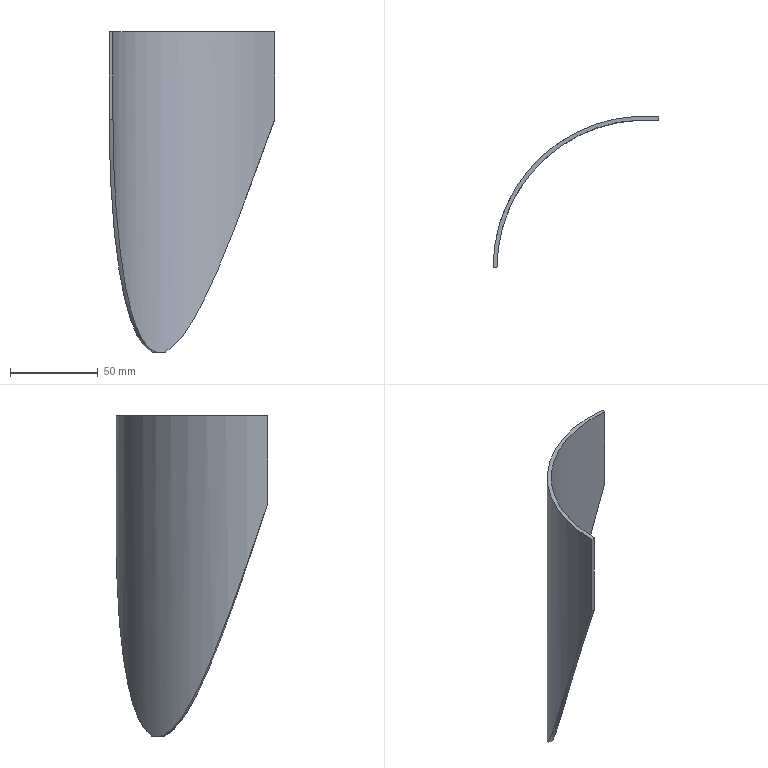Part | SolidWorks | 1 solid | 10 faces | box 94.546 x 86.364 x 182.8 mm | volume 42412 mm3 | plane 6 | cylinder 2 | spline 2 | commonest cylinder face diameters 168.269 x1 172.729 x1
STEP:
#1=CARTESIAN_POINT('',(83.843,-110.233,-985.22));
#2=VERTEX_POINT('',#1);
#3=CARTESIAN_POINT('',(83.843,-110.233,-984.858));
#4=VERTEX_POINT('',#3);
#5=CARTESIAN_POINT('',(83.843,-110.233,-985.22));
#6=DIRECTION('',(0.,0.,1.));
#7=VECTOR('',#6,1000.);
#8=LINE('',#5,#7);
#9=EDGE_CURVE('',#2,#4,#8,.T.);
#10=ORIENTED_EDGE('',*,*,#9,.F.);
#11=CARTESIAN_POINT('',(89.513,-104.991,-985.22));
#12=VERTEX_POINT('',#11);
#13=CARTESIAN_POINT('',(143.73,-169.327,-985.22));
#14=DIRECTION('',(0.,0.,-1.));
#15=DIRECTION('',(-0.7118,0.7024,0.));
#16=AXIS2_PLACEMENT_3D('',#13,#14,#15);
#17=CIRCLE('',#16,84.134);
#18=EDGE_CURVE('',#2,#12,#17,.T.);
#19=ORIENTED_EDGE('',*,*,#18,.T.);
#20=CARTESIAN_POINT('',(89.513,-104.991,-984.533));
#21=VERTEX_POINT('',#20);
#22=CARTESIAN_POINT('',(89.513,-104.991,-985.22));
#23=DIRECTION('',(0.,0.,1.));
#24=VECTOR('',#23,1000.);
#25=LINE('',#22,#24);
#26=EDGE_CURVE('',#12,#21,#25,.T.);
#27=ORIENTED_EDGE('',*,*,#26,.T.);
#28=CARTESIAN_POINT('',(151.7,-85.571,-852.42));
#29=VERTEX_POINT('',#28);
#30=CARTESIAN_POINT('',(151.7,-85.571,-852.42));
#31=CARTESIAN_POINT('',(150.614,-85.468,-855.388));
#32=CARTESIAN_POINT('',(149.545,-85.387,-858.323));
#33=CARTESIAN_POINT('',(147.407,-85.266,-864.21));
#34=CARTESIAN_POINT('',(146.334,-85.226,-867.173));
#35=CARTESIAN_POINT('',(144.195,-85.187,-873.077));
#36=CARTESIAN_POINT('',(143.126,-85.188,-876.029));
#37=CARTESIAN_POINT('',(140.983,-85.231,-881.932));
#38=CARTESIAN_POINT('',(139.91,-85.272,-884.884));
#39=CARTESIAN_POINT('',(136.678,-85.461,-893.73));
#40=CARTESIAN_POINT('',(134.508,-85.67,-899.62));
#41=CARTESIAN_POINT('',(130.095,-86.275,-911.365));
#42=CARTESIAN_POINT('',(127.853,-86.67,-917.219));
#43=CARTESIAN_POINT('',(124.395,-87.436,-925.949));
#44=CARTESIAN_POINT('',(123.226,-87.72,-928.851));
#45=CARTESIAN_POINT('',(121.442,-88.196,-933.183));
#46=CARTESIAN_POINT('',(120.842,-88.363,-934.624));
#47=CARTESIAN_POINT('',(119.629,-88.716,-937.501));
#48=CARTESIAN_POINT('',(119.018,-88.901,-938.933));
#49=CARTESIAN_POINT('',(118.089,-89.194,-941.078));
#50=CARTESIAN_POINT('',(117.778,-89.294,-941.792));
#51=CARTESIAN_POINT('',(117.152,-89.5,-943.216));
#52=CARTESIAN_POINT('',(116.838,-89.605,-943.926));
#53=CARTESIAN_POINT('',(115.887,-89.93,-946.056));
#54=CARTESIAN_POINT('',(115.243,-90.159,-947.475));
#55=CARTESIAN_POINT('',(113.942,-90.639,-950.291));
#56=CARTESIAN_POINT('',(113.282,-90.892,-951.691));
#57=CARTESIAN_POINT('',(111.94,-91.426,-954.479));
#58=CARTESIAN_POINT('',(111.258,-91.708,-955.867));
#59=CARTESIAN_POINT('',(109.868,-92.304,-958.619));
#60=CARTESIAN_POINT('',(109.161,-92.618,-959.985));
#61=CARTESIAN_POINT('',(107.716,-93.286,-962.691));
#62=CARTESIAN_POINT('',(106.978,-93.639,-964.033));
#63=CARTESIAN_POINT('',(105.465,-94.393,-966.68));
#64=CARTESIAN_POINT('',(104.69,-94.793,-967.986));
#65=CARTESIAN_POINT('',(103.096,-95.65,-970.553));
#66=CARTESIAN_POINT('',(102.276,-96.107,-971.813));
#67=CARTESIAN_POINT('',(100.581,-97.093,-974.266));
#68=CARTESIAN_POINT('',(99.706,-97.621,-975.458));
#69=CARTESIAN_POINT('',(97.884,-98.772,-977.745));
#70=CARTESIAN_POINT('',(96.94,-99.393,-978.838));
#71=CARTESIAN_POINT('',(94.965,-100.756,-980.866));
#72=CARTESIAN_POINT('',(93.934,-101.498,-981.799));
#73=CARTESIAN_POINT('',(91.783,-103.13,-983.404));
#74=CARTESIAN_POINT('',(90.662,-104.023,-984.073));
#75=CARTESIAN_POINT('',(89.513,-104.991,-984.533));
#76=B_SPLINE_CURVE_WITH_KNOTS('',3,(#30,#31,#32,#33,#34,#35,#36,#37,#38,#39,#40,#41,#42,#43,#44,#45,#46,#47,#48,#49,#50,#51,#52,#53,#54,#55,#56,#57,#58,#59,#60,#61,#62,#63,#64,#65,#66,#67,#68,#69,#70,#71,#72,#73,#74,#75),.UNSPECIFIED.,.F.,.F.,(4,2,2,2,2,2,2,2,2,2,2,2,2,2,2,2,2,2,2,2,2,2,4),(0.,0.0625,0.125,0.1875,0.25,0.375,0.5,0.5625,0.5938,0.625,0.6406,0.6563,0.6875,0.7188,0.75,0.7813,0.8125,0.8438,0.875,0.9063,0.9375,0.9688,1.),.UNSPECIFIED.);
#77=EDGE_CURVE('',#29,#21,#76,.T.);
#78=ORIENTED_EDGE('',*,*,#77,.F.);
#79=CARTESIAN_POINT('',(151.7,-85.571,-802.42));
#80=VERTEX_POINT('',#79);
#81=CARTESIAN_POINT('',(151.7,-85.571,-802.42));
#82=DIRECTION('',(0.,0.,-1.));
#83=VECTOR('',#82,1000.);
#84=LINE('',#81,#83);
#85=EDGE_CURVE('',#80,#29,#84,.T.);
#86=ORIENTED_EDGE('',*,*,#85,.F.);
#87=CARTESIAN_POINT('',(59.595,-169.327,-802.42));
#88=VERTEX_POINT('',#87);
#89=CARTESIAN_POINT('',(143.73,-169.327,-802.42));
#90=DIRECTION('',(0.,0.,1.));
#91=DIRECTION('',(0.09473,0.9955,0.));
#92=AXIS2_PLACEMENT_3D('',#89,#90,#91);
#93=CIRCLE('',#92,84.134);
#94=EDGE_CURVE('',#80,#88,#93,.T.);
#95=ORIENTED_EDGE('',*,*,#94,.T.);
#96=CARTESIAN_POINT('',(59.595,-169.327,-852.42));
#97=VERTEX_POINT('',#96);
#98=CARTESIAN_POINT('',(59.595,-169.327,-852.42));
#99=DIRECTION('',(0.,0.,1.));
#100=VECTOR('',#99,1000.);
#101=LINE('',#98,#100);
#102=EDGE_CURVE('',#97,#88,#101,.T.);
#103=ORIENTED_EDGE('',*,*,#102,.F.);
#104=CARTESIAN_POINT('',(83.843,-110.233,-984.858));
#105=CARTESIAN_POINT('',(83.303,-110.78,-984.687));
#106=CARTESIAN_POINT('',(82.781,-111.324,-984.458));
#107=CARTESIAN_POINT('',(81.775,-112.399,-983.902));
#108=CARTESIAN_POINT('',(81.293,-112.929,-983.575));
#109=CARTESIAN_POINT('',(79.905,-114.491,-982.478));
#110=CARTESIAN_POINT('',(79.06,-115.494,-981.595));
#111=CARTESIAN_POINT('',(77.509,-117.414,-979.643));
#112=CARTESIAN_POINT('',(76.802,-118.332,-978.575));
#113=CARTESIAN_POINT('',(75.491,-120.1,-976.326));
#114=CARTESIAN_POINT('',(74.888,-120.949,-975.145));
#115=CARTESIAN_POINT('',(73.763,-122.59,-972.708));
#116=CARTESIAN_POINT('',(73.241,-123.384,-971.451));
#117=CARTESIAN_POINT('',(72.261,-124.923,-968.89));
#118=CARTESIAN_POINT('',(71.803,-125.67,-967.584));
#119=CARTESIAN_POINT('',(70.938,-127.128,-964.932));
#120=CARTESIAN_POINT('',(70.532,-127.838,-963.589));
#121=CARTESIAN_POINT('',(69.762,-129.228,-960.874));
#122=CARTESIAN_POINT('',(69.397,-129.908,-959.501));
#123=CARTESIAN_POINT('',(68.705,-131.242,-956.737));
#124=CARTESIAN_POINT('',(68.378,-131.894,-955.348));
#125=CARTESIAN_POINT('',(67.753,-133.179,-952.548));
#126=CARTESIAN_POINT('',(67.455,-133.813,-951.134));
#127=CARTESIAN_POINT('',(66.603,-135.682,-946.886));
#128=CARTESIAN_POINT('',(66.089,-136.89,-944.029));
#129=CARTESIAN_POINT('',(64.671,-140.433,-935.396));
#130=CARTESIAN_POINT('',(63.892,-142.685,-929.572));
#131=CARTESIAN_POINT('',(62.563,-147.059,-917.849));
#132=CARTESIAN_POINT('',(62.015,-149.179,-911.951));
#133=CARTESIAN_POINT('',(61.101,-153.34,-900.111));
#134=CARTESIAN_POINT('',(60.734,-155.38,-894.17));
#135=CARTESIAN_POINT('',(60.156,-159.413,-882.267));
#136=CARTESIAN_POINT('',(59.945,-161.407,-876.302));
#137=CARTESIAN_POINT('',(59.77,-163.886,-868.844));
#138=CARTESIAN_POINT('',(59.739,-164.382,-867.35));
#139=CARTESIAN_POINT('',(59.687,-165.374,-864.36));
#140=CARTESIAN_POINT('',(59.665,-165.869,-862.865));
#141=CARTESIAN_POINT('',(59.613,-167.349,-858.395));
#142=CARTESIAN_POINT('',(59.596,-168.332,-855.424));
#143=CARTESIAN_POINT('',(59.595,-169.327,-852.42));
#144=B_SPLINE_CURVE_WITH_KNOTS('',3,(#104,#105,#106,#107,#108,#109,#110,#111,#112,#113,#114,#115,#116,#117,#118,#119,#120,#121,#122,#123,#124,#125,#126,#127,#128,#129,#130,#131,#132,#133,#134,#135,#136,#137,#138,#139,#140,#141,#142,#143),.UNSPECIFIED.,.F.,.F.,(4,2,2,2,2,2,2,2,2,2,2,2,2,2,2,2,2,2,2,4),(0.,0.01563,0.03125,0.0625,0.09375,0.125,0.1563,0.1875,0.2188,0.25,0.2813,0.3125,0.375,0.5,0.625,0.75,0.875,0.9063,0.9375,1.),.UNSPECIFIED.);
#145=EDGE_CURVE('',#4,#97,#144,.T.);
#146=ORIENTED_EDGE('',*,*,#145,.F.);
#147=EDGE_LOOP('',(#10,#19,#27,#78,#86,#95,#103,#146));
#148=FACE_OUTER_BOUND('',#147,.T.);
#149=CARTESIAN_POINT('',(143.73,-169.327,-802.42));
#150=DIRECTION('',(0.,0.,-1.));
#151=DIRECTION('',(-1.,0.,0.));
#152=AXIS2_PLACEMENT_3D('',#149,#150,#151);
#153=CYLINDRICAL_SURFACE('',#152,84.134);
#154=ADVANCED_FACE('',(#148),#153,.F.);
#155=CARTESIAN_POINT('',(82.255,-108.666,-985.22));
#156=VERTEX_POINT('',#155);
#157=CARTESIAN_POINT('',(82.255,-108.666,-985.22));
#158=DIRECTION('',(0.7118,-0.7024,0.));
#159=VECTOR('',#158,1000.);
#160=LINE('',#157,#159);
#161=EDGE_CURVE('',#156,#2,#160,.T.);
#162=ORIENTED_EDGE('',*,*,#161,.T.);
#163=ORIENTED_EDGE('',*,*,#9,.T.);
#164=CARTESIAN_POINT('',(82.255,-108.666,-984.858));
#165=VERTEX_POINT('',#164);
#166=CARTESIAN_POINT('',(83.049,-109.45,-984.858));
#167=DIRECTION('',(-0.7118,0.7024,0.));
#168=VECTOR('',#167,1000.);
#169=LINE('',#166,#168);
#170=EDGE_CURVE('',#4,#165,#169,.T.);
#171=ORIENTED_EDGE('',*,*,#170,.T.);
#172=CARTESIAN_POINT('',(82.255,-108.666,-984.858));
#173=DIRECTION('',(0.,0.,-1.));
#174=VECTOR('',#173,1000.);
#175=LINE('',#172,#174);
#176=EDGE_CURVE('',#165,#156,#175,.T.);
#177=ORIENTED_EDGE('',*,*,#176,.T.);
#178=EDGE_LOOP('',(#162,#163,#171,#177));
#179=FACE_OUTER_BOUND('',#178,.T.);
#180=CARTESIAN_POINT('',(83.049,-109.45,-985.039));
#181=DIRECTION('',(0.7024,0.7118,0.));
#182=DIRECTION('',(0.,0.,-1.));
#183=AXIS2_PLACEMENT_3D('',#180,#181,#182);
#184=PLANE('',#183);
#185=ADVANCED_FACE('',(#179),#184,.F.);
#186=CARTESIAN_POINT('',(88.076,-103.286,-985.22));
#187=VERTEX_POINT('',#186);
#188=CARTESIAN_POINT('',(89.513,-104.991,-985.22));
#189=DIRECTION('',(-0.6444,0.7647,0.));
#190=VECTOR('',#189,1000.);
#191=LINE('',#188,#190);
#192=EDGE_CURVE('',#12,#187,#191,.T.);
#193=ORIENTED_EDGE('',*,*,#192,.F.);
#194=ORIENTED_EDGE('',*,*,#18,.F.);
#195=ORIENTED_EDGE('',*,*,#161,.F.);
#196=CARTESIAN_POINT('',(143.73,-169.327,-985.22));
#197=DIRECTION('',(0.,0.,1.));
#198=DIRECTION('',(-0.6444,0.7647,0.));
#199=AXIS2_PLACEMENT_3D('',#196,#197,#198);
#200=CIRCLE('',#199,86.364);
#201=EDGE_CURVE('',#187,#156,#200,.T.);
#202=ORIENTED_EDGE('',*,*,#201,.F.);
#203=EDGE_LOOP('',(#193,#194,#195,#202));
#204=FACE_OUTER_BOUND('',#203,.T.);
#205=CARTESIAN_POINT('',(85.86,-106.728,-985.22));
#206=DIRECTION('',(0.,0.,1.));
#207=DIRECTION('',(0.7024,0.7118,0.));
#208=AXIS2_PLACEMENT_3D('',#205,#206,#207);
#209=PLANE('',#208);
#210=ADVANCED_FACE('',(#204),#209,.F.);
#211=CARTESIAN_POINT('',(88.076,-103.286,-984.533));
#212=VERTEX_POINT('',#211);
#213=CARTESIAN_POINT('',(88.794,-104.138,-984.533));
#214=DIRECTION('',(0.6444,-0.7647,0.));
#215=VECTOR('',#214,1000.);
#216=LINE('',#213,#215);
#217=EDGE_CURVE('',#212,#21,#216,.T.);
#218=ORIENTED_EDGE('',*,*,#217,.T.);
#219=ORIENTED_EDGE('',*,*,#26,.F.);
#220=ORIENTED_EDGE('',*,*,#192,.T.);
#221=CARTESIAN_POINT('',(88.076,-103.286,-985.22));
#222=DIRECTION('',(0.,0.,1.));
#223=VECTOR('',#222,1000.);
#224=LINE('',#221,#223);
#225=EDGE_CURVE('',#187,#212,#224,.T.);
#226=ORIENTED_EDGE('',*,*,#225,.T.);
#227=EDGE_LOOP('',(#218,#219,#220,#226));
#228=FACE_OUTER_BOUND('',#227,.T.);
#229=CARTESIAN_POINT('',(88.794,-104.138,-984.877));
#230=DIRECTION('',(0.7647,0.6444,0.));
#231=DIRECTION('',(0.,0.,-1.));
#232=AXIS2_PLACEMENT_3D('',#229,#230,#231);
#233=PLANE('',#232);
#234=ADVANCED_FACE('',(#228),#233,.T.);
#235=CARTESIAN_POINT('',(151.911,-83.351,-852.42));
#236=VERTEX_POINT('',#235);
#237=CARTESIAN_POINT('',(151.805,-84.461,-852.42));
#238=DIRECTION('',(0.09473,0.9955,0.));
#239=VECTOR('',#238,1000.);
#240=LINE('',#237,#239);
#241=EDGE_CURVE('',#29,#236,#240,.T.);
#242=ORIENTED_EDGE('',*,*,#241,.F.);
#243=ORIENTED_EDGE('',*,*,#77,.T.);
#244=ORIENTED_EDGE('',*,*,#217,.F.);
#245=CARTESIAN_POINT('',(88.076,-103.286,-984.533));
#246=CARTESIAN_POINT('',(89.234,-102.31,-984.082));
#247=CARTESIAN_POINT('',(90.367,-101.407,-983.427));
#248=CARTESIAN_POINT('',(92.548,-99.749,-981.852));
#249=CARTESIAN_POINT('',(93.596,-98.993,-980.935));
#250=CARTESIAN_POINT('',(95.609,-97.601,-978.936));
#251=CARTESIAN_POINT('',(96.573,-96.965,-977.856));
#252=CARTESIAN_POINT('',(98.436,-95.785,-975.591));
#253=CARTESIAN_POINT('',(99.332,-95.241,-974.408));
#254=CARTESIAN_POINT('',(101.068,-94.228,-971.972));
#255=CARTESIAN_POINT('',(101.909,-93.758,-970.719));
#256=CARTESIAN_POINT('',(103.545,-92.875,-968.166));
#257=CARTESIAN_POINT('',(104.34,-92.463,-966.864));
#258=CARTESIAN_POINT('',(105.893,-91.687,-964.225));
#259=CARTESIAN_POINT('',(106.652,-91.322,-962.887));
#260=CARTESIAN_POINT('',(108.137,-90.634,-960.186));
#261=CARTESIAN_POINT('',(108.863,-90.309,-958.823));
#262=CARTESIAN_POINT('',(110.292,-89.694,-956.073));
#263=CARTESIAN_POINT('',(110.993,-89.404,-954.687));
#264=CARTESIAN_POINT('',(112.374,-88.852,-951.9));
#265=CARTESIAN_POINT('',(113.052,-88.591,-950.499));
#266=CARTESIAN_POINT('',(114.391,-88.096,-947.684));
#267=CARTESIAN_POINT('',(115.052,-87.86,-946.266));
#268=CARTESIAN_POINT('',(116.357,-87.412,-943.421));
#269=CARTESIAN_POINT('',(117.,-87.2,-941.998));
#270=CARTESIAN_POINT('',(118.274,-86.797,-939.135));
#271=CARTESIAN_POINT('',(118.903,-86.605,-937.702));
#272=CARTESIAN_POINT('',(120.15,-86.241,-934.821));
#273=CARTESIAN_POINT('',(120.768,-86.068,-933.378));
#274=CARTESIAN_POINT('',(122.603,-85.577,-929.04));
#275=CARTESIAN_POINT('',(123.807,-85.283,-926.133));
#276=CARTESIAN_POINT('',(127.366,-84.492,-917.386));
#277=CARTESIAN_POINT('',(129.673,-84.083,-911.519));
#278=CARTESIAN_POINT('',(134.216,-83.458,-899.747));
#279=CARTESIAN_POINT('',(136.45,-83.241,-893.84));
#280=CARTESIAN_POINT('',(140.885,-82.981,-882.015));
#281=CARTESIAN_POINT('',(143.086,-82.937,-876.093));
#282=CARTESIAN_POINT('',(146.388,-82.996,-867.212));
#283=CARTESIAN_POINT('',(147.492,-83.037,-864.242));
#284=CARTESIAN_POINT('',(149.694,-83.162,-858.337));
#285=CARTESIAN_POINT('',(150.794,-83.245,-855.394));
#286=CARTESIAN_POINT('',(151.911,-83.351,-852.42));
#287=B_SPLINE_CURVE_WITH_KNOTS('',3,(#245,#246,#247,#248,#249,#250,#251,#252,#253,#254,#255,#256,#257,#258,#259,#260,#261,#262,#263,#264,#265,#266,#267,#268,#269,#270,#271,#272,#273,#274,#275,#276,#277,#278,#279,#280,#281,#282,#283,#284,#285,#286),.UNSPECIFIED.,.F.,.F.,(4,2,2,2,2,2,2,2,2,2,2,2,2,2,2,2,2,2,2,2,4),(0.,0.03125,0.0625,0.09375,0.125,0.1563,0.1875,0.2188,0.25,0.2813,0.3125,0.3438,0.375,0.4063,0.4375,0.5,0.625,0.75,0.875,0.9375,1.),.UNSPECIFIED.);
#288=EDGE_CURVE('',#212,#236,#287,.T.);
#289=ORIENTED_EDGE('',*,*,#288,.T.);
#290=EDGE_LOOP('',(#242,#243,#244,#289));
#291=FACE_OUTER_BOUND('',#290,.T.);
#292=CARTESIAN_POINT('',(152.469,-83.136,-851.006));
#293=CARTESIAN_POINT('',(152.376,-84.053,-851.006));
#294=CARTESIAN_POINT('',(152.283,-84.971,-851.006));
#295=CARTESIAN_POINT('',(152.19,-85.889,-851.006));
#296=CARTESIAN_POINT('',(152.292,-83.118,-851.477));
#297=CARTESIAN_POINT('',(152.201,-84.036,-851.477));
#298=CARTESIAN_POINT('',(152.109,-84.954,-851.477));
#299=CARTESIAN_POINT('',(152.018,-85.871,-851.477));
#300=CARTESIAN_POINT('',(150.752,-82.967,-855.56));
#301=CARTESIAN_POINT('',(150.677,-83.886,-855.56));
#302=CARTESIAN_POINT('',(150.603,-84.806,-855.56));
#303=CARTESIAN_POINT('',(150.528,-85.725,-855.56));
#304=CARTESIAN_POINT('',(147.847,-82.758,-863.317));
#305=CARTESIAN_POINT('',(147.803,-83.68,-863.317));
#306=CARTESIAN_POINT('',(147.759,-84.601,-863.317));
#307=CARTESIAN_POINT('',(147.716,-85.523,-863.317));
#308=CARTESIAN_POINT('',(143.616,-82.66,-874.671));
#309=CARTESIAN_POINT('',(143.617,-83.583,-874.671));
#310=CARTESIAN_POINT('',(143.618,-84.505,-874.671));
#311=CARTESIAN_POINT('',(143.619,-85.428,-874.671));
#312=CARTESIAN_POINT('',(139.544,-82.766,-885.568));
#313=CARTESIAN_POINT('',(139.589,-83.687,-885.568));
#314=CARTESIAN_POINT('',(139.633,-84.609,-885.568));
#315=CARTESIAN_POINT('',(139.678,-85.53,-885.568));
#316=CARTESIAN_POINT('',(135.85,-83.03,-895.364));
#317=CARTESIAN_POINT('',(135.934,-83.949,-895.364));
#318=CARTESIAN_POINT('',(136.018,-84.867,-895.364));
#319=CARTESIAN_POINT('',(136.102,-85.786,-895.364));
#320=CARTESIAN_POINT('',(132.603,-83.392,-903.857));
#321=CARTESIAN_POINT('',(132.721,-84.307,-903.857));
#322=CARTESIAN_POINT('',(132.84,-85.222,-903.857));
#323=CARTESIAN_POINT('',(132.958,-86.137,-903.857));
#324=CARTESIAN_POINT('',(129.554,-83.844,-911.696));
#325=CARTESIAN_POINT('',(129.705,-84.754,-911.696));
#326=CARTESIAN_POINT('',(129.856,-85.664,-911.696));
#327=CARTESIAN_POINT('',(130.007,-86.575,-911.696));
#328=CARTESIAN_POINT('',(126.746,-84.36,-918.768));
#329=CARTESIAN_POINT('',(126.927,-85.265,-918.768));
#330=CARTESIAN_POINT('',(127.108,-86.169,-918.768));
#331=CARTESIAN_POINT('',(127.289,-87.074,-918.768));
#332=CARTESIAN_POINT('',(124.157,-84.921,-925.14));
#333=CARTESIAN_POINT('',(124.366,-85.82,-925.14));
#334=CARTESIAN_POINT('',(124.574,-86.718,-925.14));
#335=CARTESIAN_POINT('',(124.782,-87.617,-925.14));
#336=CARTESIAN_POINT('',(121.795,-85.506,-930.81));
#337=CARTESIAN_POINT('',(122.028,-86.399,-930.81));
#338=CARTESIAN_POINT('',(122.262,-87.291,-930.81));
#339=CARTESIAN_POINT('',(122.496,-88.183,-930.81));
#340=CARTESIAN_POINT('',(119.681,-86.09,-935.751));
#341=CARTESIAN_POINT('',(119.938,-86.976,-935.751));
#342=CARTESIAN_POINT('',(120.194,-87.862,-935.751));
#343=CARTESIAN_POINT('',(120.45,-88.748,-935.751));
#344=CARTESIAN_POINT('',(117.732,-86.678,-940.192));
#345=CARTESIAN_POINT('',(118.009,-87.558,-940.192));
#346=CARTESIAN_POINT('',(118.286,-88.438,-940.192));
#347=CARTESIAN_POINT('',(118.562,-89.318,-940.192));
#348=CARTESIAN_POINT('',(115.769,-87.321,-944.539));
#349=CARTESIAN_POINT('',(116.066,-88.194,-944.539));
#350=CARTESIAN_POINT('',(116.364,-89.067,-944.539));
#351=CARTESIAN_POINT('',(116.662,-89.94,-944.539));
#352=CARTESIAN_POINT('',(113.692,-88.057,-948.986));
#353=CARTESIAN_POINT('',(114.012,-88.923,-948.986));
#354=CARTESIAN_POINT('',(114.332,-89.788,-948.986));
#355=CARTESIAN_POINT('',(114.652,-90.653,-948.986));
#356=CARTESIAN_POINT('',(111.544,-88.883,-953.407));
#357=CARTESIAN_POINT('',(111.887,-89.739,-953.407));
#358=CARTESIAN_POINT('',(112.23,-90.596,-953.407));
#359=CARTESIAN_POINT('',(112.572,-91.452,-953.407));
#360=CARTESIAN_POINT('',(109.338,-89.8,-957.742));
#361=CARTESIAN_POINT('',(109.704,-90.647,-957.742));
#362=CARTESIAN_POINT('',(110.07,-91.494,-957.742));
#363=CARTESIAN_POINT('',(110.436,-92.341,-957.742));
#364=CARTESIAN_POINT('',(107.093,-90.809,-961.921));
#365=CARTESIAN_POINT('',(107.483,-91.645,-961.921));
#366=CARTESIAN_POINT('',(107.873,-92.481,-961.921));
#367=CARTESIAN_POINT('',(108.263,-93.317,-961.921));
#368=CARTESIAN_POINT('',(104.829,-91.905,-965.874));
#369=CARTESIAN_POINT('',(105.243,-92.729,-965.874));
#370=CARTESIAN_POINT('',(105.657,-93.554,-965.874));
#371=CARTESIAN_POINT('',(106.071,-94.378,-965.874));
#372=CARTESIAN_POINT('',(102.594,-93.069,-969.5));
#373=CARTESIAN_POINT('',(103.031,-93.881,-969.5));
#374=CARTESIAN_POINT('',(103.469,-94.693,-969.5));
#375=CARTESIAN_POINT('',(103.907,-95.505,-969.5));
#376=CARTESIAN_POINT('',(100.388,-94.3,-972.787));
#377=CARTESIAN_POINT('',(100.85,-95.099,-972.787));
#378=CARTESIAN_POINT('',(101.311,-95.898,-972.787));
#379=CARTESIAN_POINT('',(101.773,-96.697,-972.787));
#380=CARTESIAN_POINT('',(98.152,-95.636,-975.803));
#381=CARTESIAN_POINT('',(98.637,-96.421,-975.803));
#382=CARTESIAN_POINT('',(99.122,-97.205,-975.803));
#383=CARTESIAN_POINT('',(99.607,-97.99,-975.803));
#384=CARTESIAN_POINT('',(95.801,-97.141,-978.599));
#385=CARTESIAN_POINT('',(96.311,-97.909,-978.599));
#386=CARTESIAN_POINT('',(96.821,-98.678,-978.599));
#387=CARTESIAN_POINT('',(97.331,-99.446,-978.599));
#388=CARTESIAN_POINT('',(93.314,-98.851,-981.099));
#389=CARTESIAN_POINT('',(93.851,-99.601,-981.099));
#390=CARTESIAN_POINT('',(94.388,-100.351,-981.099));
#391=CARTESIAN_POINT('',(94.925,-101.102,-981.099));
#392=CARTESIAN_POINT('',(90.661,-100.822,-983.191));
#393=CARTESIAN_POINT('',(91.226,-101.551,-983.191));
#394=CARTESIAN_POINT('',(91.791,-102.281,-983.191));
#395=CARTESIAN_POINT('',(92.356,-103.01,-983.191));
#396=CARTESIAN_POINT('',(88.473,-102.586,-984.365));
#397=CARTESIAN_POINT('',(89.061,-103.297,-984.365));
#398=CARTESIAN_POINT('',(89.65,-104.007,-984.365));
#399=CARTESIAN_POINT('',(90.238,-104.718,-984.365));
#400=CARTESIAN_POINT('',(87.155,-103.716,-984.802));
#401=CARTESIAN_POINT('',(87.757,-104.414,-984.802));
#402=CARTESIAN_POINT('',(88.36,-105.113,-984.802));
#403=CARTESIAN_POINT('',(88.962,-105.811,-984.802));
#404=CARTESIAN_POINT('',(86.775,-104.046,-984.906));
#405=CARTESIAN_POINT('',(87.382,-104.741,-984.906));
#406=CARTESIAN_POINT('',(87.988,-105.436,-984.906));
#407=CARTESIAN_POINT('',(88.595,-106.132,-984.906));
#408=B_SPLINE_SURFACE_WITH_KNOTS('',3,3,((#292,#293,#294,#295),(#296,#297,#298,#299),(#300,#301,#302,#303),(#304,#305,#306,#307),(#308,#309,#310,#311),(#312,#313,#314,#315),(#316,#317,#318,#319),(#320,#321,#322,#323),(#324,#325,#326,#327),(#328,#329,#330,#331),(#332,#333,#334,#335),(#336,#337,#338,#339),(#340,#341,#342,#343),(#344,#345,#346,#347),(#348,#349,#350,#351),(#352,#353,#354,#355),(#356,#357,#358,#359),(#360,#361,#362,#363),(#364,#365,#366,#367),(#368,#369,#370,#371),(#372,#373,#374,#375),(#376,#377,#378,#379),(#380,#381,#382,#383),(#384,#385,#386,#387),(#388,#389,#390,#391),(#392,#393,#394,#395),(#396,#397,#398,#399),(#400,#401,#402,#403),(#404,#405,#406,#407)),.UNSPECIFIED.,.F.,.F.,.F.,(4,1,1,1,1,1,1,1,1,1,1,1,1,1,1,1,1,1,1,1,1,1,1,1,1,1,4),(4,4),(-0.005438,0.,0.04167,0.08333,0.125,0.1667,0.2083,0.25,0.2917,0.3333,0.375,0.4167,0.4583,0.5,0.5417,0.5833,0.625,0.6667,0.7083,0.75,0.7917,0.8333,0.875,0.9167,0.9583,1.,1.017),(-0.00003046,1.),.UNSPECIFIED.);
#409=ADVANCED_FACE('',(#291),#408,.F.);
#410=CARTESIAN_POINT('',(151.911,-83.351,-802.42));
#411=VERTEX_POINT('',#410);
#412=CARTESIAN_POINT('',(151.911,-83.351,-802.42));
#413=DIRECTION('',(-0.09473,-0.9955,0.));
#414=VECTOR('',#413,1000.);
#415=LINE('',#412,#414);
#416=EDGE_CURVE('',#411,#80,#415,.T.);
#417=ORIENTED_EDGE('',*,*,#416,.T.);
#418=ORIENTED_EDGE('',*,*,#85,.T.);
#419=ORIENTED_EDGE('',*,*,#241,.T.);
#420=CARTESIAN_POINT('',(151.911,-83.351,-852.42));
#421=DIRECTION('',(0.,0.,1.));
#422=VECTOR('',#421,1000.);
#423=LINE('',#420,#422);
#424=EDGE_CURVE('',#236,#411,#423,.T.);
#425=ORIENTED_EDGE('',*,*,#424,.T.);
#426=EDGE_LOOP('',(#417,#418,#419,#425));
#427=FACE_OUTER_BOUND('',#426,.T.);
#428=CARTESIAN_POINT('',(151.805,-84.461,-827.42));
#429=DIRECTION('',(0.9955,-0.09473,0.));
#430=DIRECTION('',(0.,0.,-1.));
#431=AXIS2_PLACEMENT_3D('',#428,#429,#430);
#432=PLANE('',#431);
#433=ADVANCED_FACE('',(#427),#432,.T.);
#434=CARTESIAN_POINT('',(57.365,-169.327,-802.42));
#435=VERTEX_POINT('',#434);
#436=CARTESIAN_POINT('',(57.365,-169.327,-802.42));
#437=DIRECTION('',(1.,0.,0.));
#438=VECTOR('',#437,1000.);
#439=LINE('',#436,#438);
#440=EDGE_CURVE('',#435,#88,#439,.T.);
#441=ORIENTED_EDGE('',*,*,#440,.T.);
#442=ORIENTED_EDGE('',*,*,#94,.F.);
#443=ORIENTED_EDGE('',*,*,#416,.F.);
#444=CARTESIAN_POINT('',(143.73,-169.327,-802.42));
#445=DIRECTION('',(0.,0.,-1.));
#446=DIRECTION('',(-1.,0.,0.));
#447=AXIS2_PLACEMENT_3D('',#444,#445,#446);
#448=CIRCLE('',#447,86.364);
#449=EDGE_CURVE('',#435,#411,#448,.T.);
#450=ORIENTED_EDGE('',*,*,#449,.F.);
#451=EDGE_LOOP('',(#441,#442,#443,#450));
#452=FACE_OUTER_BOUND('',#451,.T.);
#453=CARTESIAN_POINT('',(86.375,-106.256,-802.42));
#454=DIRECTION('',(0.,0.,1.));
#455=DIRECTION('',(0.,1.,0.));
#456=AXIS2_PLACEMENT_3D('',#453,#454,#455);
#457=PLANE('',#456);
#458=ADVANCED_FACE('',(#452),#457,.T.);
#459=CARTESIAN_POINT('',(57.365,-169.327,-852.42));
#460=VERTEX_POINT('',#459);
#461=CARTESIAN_POINT('',(58.48,-169.327,-852.42));
#462=DIRECTION('',(1.,0.,0.));
#463=VECTOR('',#462,1000.);
#464=LINE('',#461,#463);
#465=EDGE_CURVE('',#460,#97,#464,.T.);
#466=ORIENTED_EDGE('',*,*,#465,.T.);
#467=ORIENTED_EDGE('',*,*,#102,.T.);
#468=ORIENTED_EDGE('',*,*,#440,.F.);
#469=CARTESIAN_POINT('',(57.365,-169.327,-802.42));
#470=DIRECTION('',(0.,0.,-1.));
#471=VECTOR('',#470,1000.);
#472=LINE('',#469,#471);
#473=EDGE_CURVE('',#435,#460,#472,.T.);
#474=ORIENTED_EDGE('',*,*,#473,.T.);
#475=EDGE_LOOP('',(#466,#467,#468,#474));
#476=FACE_OUTER_BOUND('',#475,.T.);
#477=CARTESIAN_POINT('',(58.48,-169.327,-827.42));
#478=DIRECTION('',(0.,1.,0.));
#479=DIRECTION('',(0.,0.,-1.));
#480=AXIS2_PLACEMENT_3D('',#477,#478,#479);
#481=PLANE('',#480);
#482=ADVANCED_FACE('',(#476),#481,.F.);
#483=ORIENTED_EDGE('',*,*,#170,.F.);
#484=ORIENTED_EDGE('',*,*,#145,.T.);
#485=ORIENTED_EDGE('',*,*,#465,.F.);
#486=CARTESIAN_POINT('',(57.365,-169.327,-852.42));
#487=CARTESIAN_POINT('',(57.366,-168.303,-855.432));
#488=CARTESIAN_POINT('',(57.383,-167.291,-858.413));
#489=CARTESIAN_POINT('',(57.437,-165.767,-862.898));
#490=CARTESIAN_POINT('',(57.46,-165.257,-864.396));
#491=CARTESIAN_POINT('',(57.514,-164.236,-867.396));
#492=CARTESIAN_POINT('',(57.546,-163.725,-868.894));
#493=CARTESIAN_POINT('',(57.727,-161.172,-876.374));
#494=CARTESIAN_POINT('',(57.945,-159.12,-882.357));
#495=CARTESIAN_POINT('',(58.542,-154.967,-894.294));
#496=CARTESIAN_POINT('',(58.92,-152.867,-900.251));
#497=CARTESIAN_POINT('',(59.865,-148.583,-912.121));
#498=CARTESIAN_POINT('',(60.431,-146.399,-918.034));
#499=CARTESIAN_POINT('',(61.46,-143.023,-926.844));
#500=CARTESIAN_POINT('',(61.833,-141.88,-929.77));
#501=CARTESIAN_POINT('',(62.651,-139.55,-935.595));
#502=CARTESIAN_POINT('',(63.096,-138.364,-938.495));
#503=CARTESIAN_POINT('',(64.072,-135.933,-944.255));
#504=CARTESIAN_POINT('',(64.603,-134.69,-947.113));
#505=CARTESIAN_POINT('',(65.482,-132.767,-951.363));
#506=CARTESIAN_POINT('',(65.79,-132.115,-952.776));
#507=CARTESIAN_POINT('',(66.434,-130.794,-955.573));
#508=CARTESIAN_POINT('',(66.773,-130.122,-956.963));
#509=CARTESIAN_POINT('',(67.844,-128.065,-961.105));
#510=CARTESIAN_POINT('',(68.63,-126.642,-963.821));
#511=CARTESIAN_POINT('',(69.968,-124.396,-967.784));
#512=CARTESIAN_POINT('',(70.44,-123.629,-969.085));
#513=CARTESIAN_POINT('',(71.448,-122.05,-971.632));
#514=CARTESIAN_POINT('',(71.986,-121.236,-972.881));
#515=CARTESIAN_POINT('',(73.142,-119.555,-975.299));
#516=CARTESIAN_POINT('',(73.761,-118.686,-976.469));
#517=CARTESIAN_POINT('',(75.105,-116.879,-978.692));
#518=CARTESIAN_POINT('',(75.83,-115.942,-979.746));
#519=CARTESIAN_POINT('',(77.413,-113.987,-981.666));
#520=CARTESIAN_POINT('',(78.273,-112.968,-982.531));
#521=CARTESIAN_POINT('',(79.681,-111.387,-983.604));
#522=CARTESIAN_POINT('',(80.169,-110.851,-983.924));
#523=CARTESIAN_POINT('',(81.185,-109.766,-984.467));
#524=CARTESIAN_POINT('',(81.712,-109.217,-984.69));
#525=CARTESIAN_POINT('',(82.255,-108.666,-984.858));
#526=B_SPLINE_CURVE_WITH_KNOTS('',3,(#486,#487,#488,#489,#490,#491,#492,#493,#494,#495,#496,#497,#498,#499,#500,#501,#502,#503,#504,#505,#506,#507,#508,#509,#510,#511,#512,#513,#514,#515,#516,#517,#518,#519,#520,#521,#522,#523,#524,#525),.UNSPECIFIED.,.F.,.F.,(4,2,2,2,2,2,2,2,2,2,2,2,2,2,2,2,2,2,2,4),(0.,0.0625,0.09375,0.125,0.25,0.375,0.5,0.5625,0.625,0.6875,0.7187,0.75,0.8125,0.8437,0.875,0.9062,0.9375,0.9687,0.9844,1.),.UNSPECIFIED.);
#527=EDGE_CURVE('',#460,#165,#526,.T.);
#528=ORIENTED_EDGE('',*,*,#527,.T.);
#529=EDGE_LOOP('',(#483,#484,#485,#528));
#530=FACE_OUTER_BOUND('',#529,.T.);
#531=CARTESIAN_POINT('',(83.127,-107.419,-985.112));
#532=CARTESIAN_POINT('',(83.772,-108.078,-985.112));
#533=CARTESIAN_POINT('',(84.417,-108.737,-985.112));
#534=CARTESIAN_POINT('',(85.063,-109.396,-985.112));
#535=CARTESIAN_POINT('',(82.765,-107.774,-985.05));
#536=CARTESIAN_POINT('',(83.414,-108.429,-985.05));
#537=CARTESIAN_POINT('',(84.063,-109.084,-985.05));
#538=CARTESIAN_POINT('',(84.712,-109.74,-985.05));
#539=CARTESIAN_POINT('',(81.563,-108.971,-984.762));
#540=CARTESIAN_POINT('',(82.225,-109.614,-984.762));
#541=CARTESIAN_POINT('',(82.887,-110.257,-984.762));
#542=CARTESIAN_POINT('',(83.548,-110.899,-984.762));
#543=CARTESIAN_POINT('',(79.664,-110.978,-983.84));
#544=CARTESIAN_POINT('',(80.346,-111.599,-983.84));
#545=CARTESIAN_POINT('',(81.028,-112.22,-983.84));
#546=CARTESIAN_POINT('',(81.71,-112.841,-983.84));
#547=CARTESIAN_POINT('',(77.511,-113.437,-982.042));
#548=CARTESIAN_POINT('',(78.216,-114.032,-982.042));
#549=CARTESIAN_POINT('',(78.921,-114.627,-982.042));
#550=CARTESIAN_POINT('',(79.626,-115.222,-982.042));
#551=CARTESIAN_POINT('',(75.614,-115.77,-979.785));
#552=CARTESIAN_POINT('',(76.339,-116.34,-979.785));
#553=CARTESIAN_POINT('',(77.065,-116.91,-979.785));
#554=CARTESIAN_POINT('',(77.79,-117.48,-979.785));
#555=CARTESIAN_POINT('',(73.908,-118.018,-977.155));
#556=CARTESIAN_POINT('',(74.651,-118.564,-977.155));
#557=CARTESIAN_POINT('',(75.394,-119.11,-977.155));
#558=CARTESIAN_POINT('',(76.138,-119.656,-977.155));
#559=CARTESIAN_POINT('',(72.372,-120.178,-974.239));
#560=CARTESIAN_POINT('',(73.132,-120.702,-974.239));
#561=CARTESIAN_POINT('',(73.891,-121.225,-974.239));
#562=CARTESIAN_POINT('',(74.651,-121.748,-974.239));
#563=CARTESIAN_POINT('',(70.979,-122.267,-971.089));
#564=CARTESIAN_POINT('',(71.754,-122.768,-971.089));
#565=CARTESIAN_POINT('',(72.528,-123.269,-971.089));
#566=CARTESIAN_POINT('',(73.303,-123.77,-971.089));
#567=CARTESIAN_POINT('',(69.716,-124.282,-967.764));
#568=CARTESIAN_POINT('',(70.504,-124.762,-967.764));
#569=CARTESIAN_POINT('',(71.292,-125.242,-967.764));
#570=CARTESIAN_POINT('',(72.08,-125.721,-967.764));
#571=CARTESIAN_POINT('',(68.567,-126.229,-964.305));
#572=CARTESIAN_POINT('',(69.367,-126.688,-964.305));
#573=CARTESIAN_POINT('',(70.167,-127.147,-964.305));
#574=CARTESIAN_POINT('',(70.968,-127.605,-964.305));
#575=CARTESIAN_POINT('',(67.532,-128.089,-960.789));
#576=CARTESIAN_POINT('',(68.343,-128.528,-960.789));
#577=CARTESIAN_POINT('',(69.154,-128.967,-960.789));
#578=CARTESIAN_POINT('',(69.966,-129.406,-960.789));
#579=CARTESIAN_POINT('',(66.605,-129.851,-957.28));
#580=CARTESIAN_POINT('',(67.426,-130.272,-957.28));
#581=CARTESIAN_POINT('',(68.247,-130.692,-957.28));
#582=CARTESIAN_POINT('',(69.068,-131.112,-957.28));
#583=CARTESIAN_POINT('',(65.759,-131.551,-953.743));
#584=CARTESIAN_POINT('',(66.589,-131.954,-953.743));
#585=CARTESIAN_POINT('',(67.419,-132.356,-953.743));
#586=CARTESIAN_POINT('',(68.249,-132.758,-953.743));
#587=CARTESIAN_POINT('',(64.973,-133.219,-950.138));
#588=CARTESIAN_POINT('',(65.812,-133.603,-950.138));
#589=CARTESIAN_POINT('',(66.65,-133.987,-950.138));
#590=CARTESIAN_POINT('',(67.489,-134.372,-950.138));
#591=CARTESIAN_POINT('',(64.254,-134.832,-946.528));
#592=CARTESIAN_POINT('',(65.1,-135.199,-946.528));
#593=CARTESIAN_POINT('',(65.946,-135.567,-946.528));
#594=CARTESIAN_POINT('',(66.792,-135.934,-946.528));
#595=CARTESIAN_POINT('',(63.592,-136.4,-942.915));
#596=CARTESIAN_POINT('',(64.445,-136.75,-942.915));
#597=CARTESIAN_POINT('',(65.298,-137.101,-942.915));
#598=CARTESIAN_POINT('',(66.152,-137.451,-942.915));
#599=CARTESIAN_POINT('',(62.949,-138.01,-939.103));
#600=CARTESIAN_POINT('',(63.809,-138.343,-939.103));
#601=CARTESIAN_POINT('',(64.669,-138.676,-939.103));
#602=CARTESIAN_POINT('',(65.529,-139.01,-939.103));
#603=CARTESIAN_POINT('',(62.301,-139.731,-934.92));
#604=CARTESIAN_POINT('',(63.168,-140.046,-934.92));
#605=CARTESIAN_POINT('',(64.035,-140.361,-934.92));
#606=CARTESIAN_POINT('',(64.902,-140.676,-934.92));
#607=CARTESIAN_POINT('',(61.632,-141.637,-930.168));
#608=CARTESIAN_POINT('',(62.506,-141.932,-930.168));
#609=CARTESIAN_POINT('',(63.38,-142.227,-930.168));
#610=CARTESIAN_POINT('',(64.254,-142.521,-930.168));
#611=CARTESIAN_POINT('',(60.951,-143.739,-924.791));
#612=CARTESIAN_POINT('',(61.832,-144.011,-924.791));
#613=CARTESIAN_POINT('',(62.714,-144.284,-924.791));
#614=CARTESIAN_POINT('',(63.595,-144.556,-924.791));
#615=CARTESIAN_POINT('',(60.273,-146.039,-918.757));
#616=CARTESIAN_POINT('',(61.162,-146.287,-918.757));
#617=CARTESIAN_POINT('',(62.05,-146.535,-918.757));
#618=CARTESIAN_POINT('',(62.939,-146.783,-918.757));
#619=CARTESIAN_POINT('',(59.615,-148.534,-912.056));
#620=CARTESIAN_POINT('',(60.51,-148.756,-912.056));
#621=CARTESIAN_POINT('',(61.406,-148.977,-912.056));
#622=CARTESIAN_POINT('',(62.301,-149.198,-912.056));
#623=CARTESIAN_POINT('',(58.98,-151.28,-904.517));
#624=CARTESIAN_POINT('',(59.883,-151.472,-904.517));
#625=CARTESIAN_POINT('',(60.785,-151.664,-904.517));
#626=CARTESIAN_POINT('',(61.687,-151.856,-904.517));
#627=CARTESIAN_POINT('',(58.384,-154.327,-895.981));
#628=CARTESIAN_POINT('',(59.292,-154.486,-895.981));
#629=CARTESIAN_POINT('',(60.201,-154.646,-895.981));
#630=CARTESIAN_POINT('',(61.11,-154.806,-895.981));
#631=CARTESIAN_POINT('',(57.834,-157.846,-885.939));
#632=CARTESIAN_POINT('',(58.748,-157.968,-885.939));
#633=CARTESIAN_POINT('',(59.663,-158.09,-885.939));
#634=CARTESIAN_POINT('',(60.577,-158.212,-885.939));
#635=CARTESIAN_POINT('',(57.404,-161.685,-874.814));
#636=CARTESIAN_POINT('',(58.323,-161.767,-874.814));
#637=CARTESIAN_POINT('',(59.242,-161.848,-874.814));
#638=CARTESIAN_POINT('',(60.161,-161.929,-874.814));
#639=CARTESIAN_POINT('',(57.147,-165.623,-863.293));
#640=CARTESIAN_POINT('',(58.069,-165.662,-863.293));
#641=CARTESIAN_POINT('',(58.991,-165.702,-863.293));
#642=CARTESIAN_POINT('',(59.913,-165.741,-863.293));
#643=CARTESIAN_POINT('',(57.093,-168.266,-855.53));
#644=CARTESIAN_POINT('',(58.016,-168.278,-855.53));
#645=CARTESIAN_POINT('',(58.938,-168.289,-855.53));
#646=CARTESIAN_POINT('',(59.86,-168.3,-855.53));
#647=CARTESIAN_POINT('',(57.097,-169.652,-851.467));
#648=CARTESIAN_POINT('',(58.019,-169.648,-851.467));
#649=CARTESIAN_POINT('',(58.942,-169.645,-851.467));
#650=CARTESIAN_POINT('',(59.864,-169.641,-851.467));
#651=CARTESIAN_POINT('',(57.098,-169.814,-850.992));
#652=CARTESIAN_POINT('',(58.02,-169.809,-850.992));
#653=CARTESIAN_POINT('',(58.943,-169.803,-850.992));
#654=CARTESIAN_POINT('',(59.865,-169.798,-850.992));
#655=B_SPLINE_SURFACE_WITH_KNOTS('',3,3,((#531,#532,#533,#534),(#535,#536,#537,#538),(#539,#540,#541,#542),(#543,#544,#545,#546),(#547,#548,#549,#550),(#551,#552,#553,#554),(#555,#556,#557,#558),(#559,#560,#561,#562),(#563,#564,#565,#566),(#567,#568,#569,#570),(#571,#572,#573,#574),(#575,#576,#577,#578),(#579,#580,#581,#582),(#583,#584,#585,#586),(#587,#588,#589,#590),(#591,#592,#593,#594),(#595,#596,#597,#598),(#599,#600,#601,#602),(#603,#604,#605,#606),(#607,#608,#609,#610),(#611,#612,#613,#614),(#615,#616,#617,#618),(#619,#620,#621,#622),(#623,#624,#625,#626),(#627,#628,#629,#630),(#631,#632,#633,#634),(#635,#636,#637,#638),(#639,#640,#641,#642),(#643,#644,#645,#646),(#647,#648,#649,#650),(#651,#652,#653,#654)),.UNSPECIFIED.,.F.,.F.,.F.,(4,1,1,1,1,1,1,1,1,1,1,1,1,1,1,1,1,1,1,1,1,1,1,1,1,1,1,1,4),(4,4),(-0.01607,0.,0.03846,0.07692,0.1154,0.1538,0.1923,0.2308,0.2692,0.3077,0.3462,0.3846,0.4231,0.4615,0.5,0.5385,0.5769,0.6154,0.6538,0.6923,0.7308,0.7692,0.8077,0.8462,0.8846,0.9231,0.9615,1.,1.005),(0.000005088,1.),.UNSPECIFIED.);
#656=ADVANCED_FACE('',(#530),#655,.F.);
#657=ORIENTED_EDGE('',*,*,#473,.F.);
#658=ORIENTED_EDGE('',*,*,#449,.T.);
#659=ORIENTED_EDGE('',*,*,#424,.F.);
#660=ORIENTED_EDGE('',*,*,#288,.F.);
#661=ORIENTED_EDGE('',*,*,#225,.F.);
#662=ORIENTED_EDGE('',*,*,#201,.T.);
#663=ORIENTED_EDGE('',*,*,#176,.F.);
#664=ORIENTED_EDGE('',*,*,#527,.F.);
#665=EDGE_LOOP('',(#657,#658,#659,#660,#661,#662,#663,#664));
#666=FACE_OUTER_BOUND('',#665,.T.);
#667=CARTESIAN_POINT('',(143.73,-169.327,-802.42));
#668=DIRECTION('',(0.,0.,-1.));
#669=DIRECTION('',(-1.,0.,0.));
#670=AXIS2_PLACEMENT_3D('',#667,#668,#669);
#671=CYLINDRICAL_SURFACE('',#670,86.364);
#672=ADVANCED_FACE('',(#666),#671,.T.);
#673=CLOSED_SHELL('',(#154,#185,#210,#234,#409,#433,#458,#482,#656,#672));
#674=MANIFOLD_SOLID_BREP('',#673);
#675=CARTESIAN_POINT('',(0.,0.,0.));
#676=DIRECTION('',(0.,0.,1.));
#677=DIRECTION('',(1.,0.,0.));
#678=AXIS2_PLACEMENT_3D('',#675,#676,#677);
#679=(LENGTH_UNIT()NAMED_UNIT(*)SI_UNIT(.MILLI.,.METRE.));
#680=UNCERTAINTY_MEASURE_WITH_UNIT(LENGTH_MEASURE(0.00001),#679,'','');
#681=(NAMED_UNIT(*)PLANE_ANGLE_UNIT()SI_UNIT($,.RADIAN.));
#682=(NAMED_UNIT(*)SI_UNIT($,.STERADIAN.)SOLID_ANGLE_UNIT());
#683=(GEOMETRIC_REPRESENTATION_CONTEXT(3)GLOBAL_UNCERTAINTY_ASSIGNED_CONTEXT((#680))GLOBAL_UNIT_ASSIGNED_CONTEXT((#679,#681,#682))REPRESENTATION_CONTEXT('',''));
#684=ADVANCED_BREP_SHAPE_REPRESENTATION('',(#674,#678),#683);